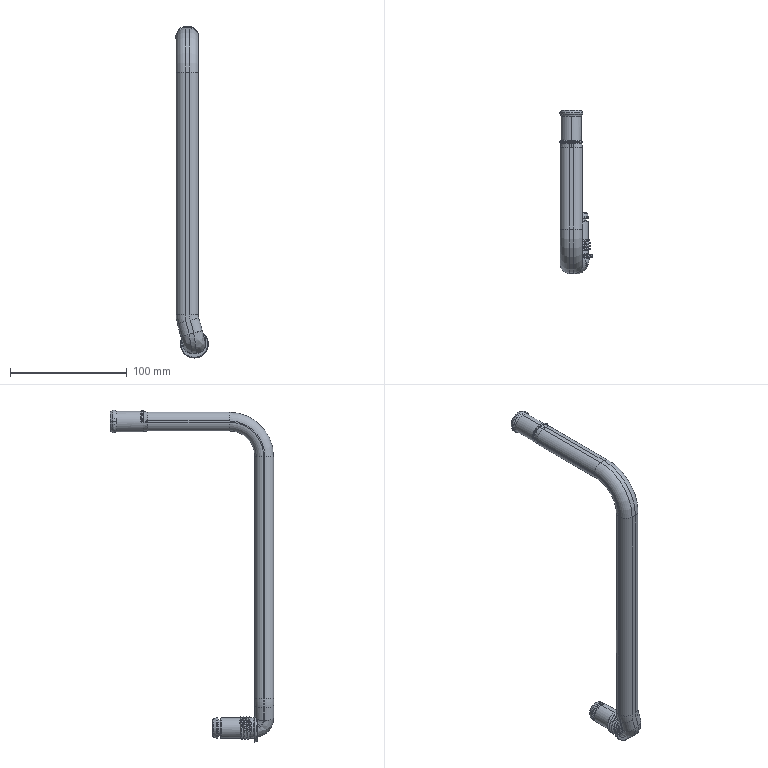Part | STEP file | ZXW722-L-19 | 1 solid | 247 faces | box 27.987 x 140.008 x 285 mm | volume 43724 mm3 | spline 101 | cylinder 59 | torus 43 | plane 28 | cone 12 | sphere 4 | commonest cylinder face diameters 11 x12 15 x12 17.2 x11 1 x8 13.6 x2 14 x2